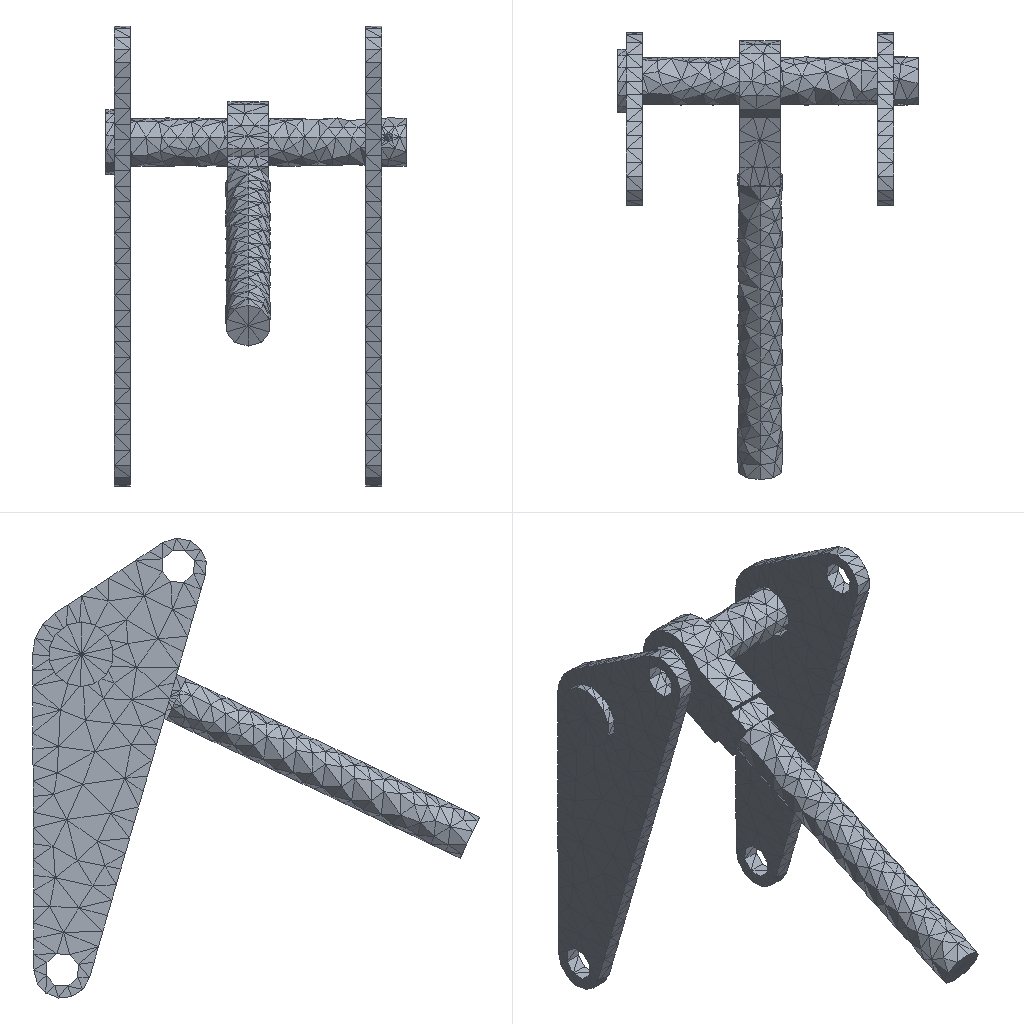Simulation study | ansys workbench
Ansys APDL input file, long lists of numbers shortened:
/batch
/config,noeldb,1     ! force off writing results to database
*get,_wallstrt,active,,time,wall
! ANSYS input file written by Workbench version 2022 R1
! File used for geometry attach:
/title,0-0--____ (C5)
! ****** Begin Custom Load Command Snippet ******
/COM, ACT Extensions:
/COM,     LSDYNA, 2021.1
/COM,
! ****** End   Custom Load Command Snippet ******
*DIM,_wb_ProjectScratch_dir,string,248
_wb_ProjectScratch_dir(1) = ''
*DIM,_wb_SolverFiles_dir,string,248
_wb_SolverFiles_dir(1) = ''
*DIM,_wb_userfiles_dir,string,248
_wb_userfiles_dir(1) = ''
/com,--- Data in consistent NMM units. See Solving Units in the help system for more information.
/units,MPA
/nopr
/wb,file,start              !  signify a WB generated input file
/prep7
! Turn off shape checking because checks already performed inside WB mesher.
! See help system for more information.
SHPP,OFF,,NOWARN
/nolist
etcon,set             ! allow ANSYS to choose best KEYOP's for 180x elements, resets any applicable keyopt to MAPDL defaults
/com,*********** Nodes for the whole assembly ***********
nblock,3,,7470
(1i9,3e20.9e3)
        1    -2.013006712E+02     4.007910257E+02    -4.722712683E+02
! (6790 more lines like these left out)
-1
/wb,elem,start            !  set before creation of elements
/com,*********** Elements for Body 1 "__28__250|____-____2" ***********
et,1,187
eblock,19,solid,,1096
(19i9)
        1        1        1        1        0        0        0        0       10        0        1       96      399      165      348     1032     1339     1025     1029
! (2191 more lines like these left out)
-1
/com,*********** Elements for Body 2 "__1|____-____1" ***********
et,2,187
eblock,19,solid,,568
(19i9)
        2        2        2        2        0        0        0        0       10        0     2588     5542     5693     5558     5617     6303     6356     6300     6302
! (1135 more lines like these left out)
-1
/com,*********** Elements for Body 3 "__1|____-____1[2]" ***********
et,3,187
eblock,19,solid,,568
(19i9)
        3        3        3        3        0        0        0        0       10        0     2020     4177     4328     4193     4252     4938     4991     4935     4937
! (1135 more lines like these left out)
-1
/com,*********** Elements for Body 4 "M30X180__|____-____1" ***********
et,4,187
eblock,19,solid,,923
(19i9)
        4        4        4        4        0        0        0        0       10        0     1097     2363     2557     2533     2548     3258     4046     3256     3257
! (1845 more lines like these left out)
-1
/wb,elem,end               !  done creating elements
/com,*********** Send User Defined Coordinate System(s) ***********
csys,0
toffst,273.15,  ! Temperature offset from absolute zero
/com,*********** Set Reference Temperature ***********
tref,22.
/wb,mat,start              !  starting to send materials
/com,*********** Send Materials ***********
Temperature = 'TEMP' ! Temperature
MP,DENS,1,7.85e-09,	! tonne mm^-3
MP,ALPX,1,1.2e-05,	! C^-1
MP,C,1,434000000,	! mm^2 s^-2 C^-1
MP,KXX,1,60.5,	! tonne mm s^-3 C^-1
MP,RSVX,1,0.00017,	! ohm mm
MP,EX,1,200000,	! tonne s^-2 mm^-1
MP,NUXY,1,0.3,
MP,MURX,1,10000,
Temperature = 'TEMP' ! Temperature
MP,DENS,2,7.85e-09,	! tonne mm^-3
MP,ALPX,2,1.2e-05,	! C^-1
MP,C,2,434000000,	! mm^2 s^-2 C^-1
MP,KXX,2,60.5,	! tonne mm s^-3 C^-1
MP,RSVX,2,0.00017,	! ohm mm
MP,EX,2,200000,	! tonne s^-2 mm^-1
MP,NUXY,2,0.3,
MP,MURX,2,10000,
Temperature = 'TEMP' ! Temperature
MP,DENS,3,7.85e-09,	! tonne mm^-3
MP,ALPX,3,1.2e-05,	! C^-1
MP,C,3,434000000,	! mm^2 s^-2 C^-1
MP,KXX,3,60.5,	! tonne mm s^-3 C^-1
MP,RSVX,3,0.00017,	! ohm mm
MP,EX,3,200000,	! tonne s^-2 mm^-1
MP,NUXY,3,0.3,
MP,MURX,3,10000,
Temperature = 'TEMP' ! Temperature
MP,DENS,4,7.85e-09,	! tonne mm^-3
MP,ALPX,4,1.2e-05,	! C^-1
MP,C,4,434000000,	! mm^2 s^-2 C^-1
MP,KXX,4,60.5,	! tonne mm s^-3 C^-1
MP,RSVX,4,0.00017,	! ohm mm
MP,EX,4,200000,	! tonne s^-2 mm^-1
MP,NUXY,4,0.3,
MP,MURX,4,10000,
/wb,mat,end                !  done sending materials
!************************* Model Summary ********************
!__28__250|____-____2,	结构钢,	matid,	1
!__1|____-____1,	结构钢,	matid,	2
!__1|____-____1[2],	结构钢,	matid,	3
!M30X180__|____-____1,	结构钢,	matid,	4
!************************* End Model Summary ********************
! get the diagonal of the bounding box. Needed later for other things
*get,_xmin,node,,mnloc,x
*get,_ymin,node,,mnloc,y
*get,_zmin,node,,mnloc,z
*get,_xmax,node,,mxloc,x
*get,_ymax,node,,mxloc,y
*get,_zmax,node,,mxloc,z
_ASMDIAG=(_xmax-_xmin)*(_xmax-_xmin)+(_ymax-_ymin)*(_ymax-_ymin)+(_zmax-_zmin)*(_zmax-_zmin)
_ASMDIAG=SQRT(_ASMDIAG)
/wb,contact,start          !  starting to send contact
/com,*********** Create Contact "摩擦的 - 杆径28行程250|____-____2 至 M30X180销轴|____-____1" ***********
/com,            Real Constant Set For Above Contact Is 6 & 5
*set,tid,6
*set,cid,5
r,tid
r,cid
et,tid,170
et,cid,174
eblock,10,,,48
(15i9)
     5424        6        6        6        0        8        9      328      328      450      462      328      453
! (47 more lines like these left out)
-1
eblock,10,,,48
(15i9)
     5472        5        5        5        0        8        9      328      328      450      462      328      453
! (47 more lines like these left out)
-1
eblock,10,,,96
(15i9)
     5520        5        6        5        0     2290     2291     2450     2450     2832     2843     2450     2836
! (95 more lines like these left out)
-1
eblock,10,,,96
(15i9)
     5616        6        5        6        0     2290     2291     2450     2450     2832     2843     2450     2836
! (95 more lines like these left out)
-1
keyo,cid,8,2               ! auto create asymmetric contact (from Program Controlled setting)
keyo,cid,10,0              ! adjust contact stiffness each NR iteration (from Program Controlled setting)
keyo,cid,12,0              ! standard contact
mp,mu,cid,0.3       ! unitless
keyo,cid,18,1              ! small sliding turned on by application
keyo,cid,2,0               ! augmented Lagrange (from Program Controlled setting)
keyo,cid,4,0               ! on Gauss point (from Program Controlled setting)
keyo,cid,9,0               ! use real geometry with stepped effects
keyo,cid,7,0               ! No Prediction
rmod,tid,3,1.       ! FKN
rmod,tid,5,0.       ! ICONT
rmod,tid,6,0.       ! PINB
rmod,tid,10,0.      ! CNOF
rmod,tid,12,0.      ! FKT
rmod,tid,36,35      ! WB DSID
rmod,cid,3,1.       ! FKN
rmod,cid,5,0.       ! ICONT
rmod,cid,6,0.       ! PINB
rmod,cid,10,0.      ! CNOF
rmod,cid,12,0.      ! FKT
rmod,cid,36,35      ! WB DSID
/com,*********** Create Contact "绑定 - M30X180销轴|____-____1 至 多个" ***********
/com,            Real Constant Set For Above Contact Is 8 & 7
*set,tid,8
*set,cid,7
r,tid
r,cid
et,tid,170
et,cid,174
eblock,10,,,404
(15i9)
     5712        8        8        8        0     2319     2318     2349     2349     3040     3043     2349     3049
! (403 more lines like these left out)
-1
eblock,10,,,404
(15i9)
     6116        7        7        7        0     2319     2318     2349     2349     3040     3043     2349     3049
! (403 more lines like these left out)
-1
eblock,10,,,48
(15i9)
     6520        7        8        7        0     5437     5439     5445     5445     5756     5771     5445     5757
! (47 more lines like these left out)
-1
eblock,10,,,48
(15i9)
     6568        8        7        8        0     5437     5439     5445     5445     5756     5771     5445     5757
! (47 more lines like these left out)
-1
keyo,cid,8,2               ! auto create asymmetric contact (from Program Controlled setting)
keyo,cid,10,0              ! adjust contact stiffness each NR iteration (from Program Controlled setting)
keyo,cid,12,5              ! bonded always
keyo,cid,2,2               ! MPC contact.  Valid only for bonded or no separation.  Requires nodal detection
keyo,cid,4,2               ! on nodal point - normal to target surface (from Program Controlled setting)
keyo,cid,9,1               ! ignore initial gaps/penetration
keyo,cid,7,0               ! No Prediction
rmod,tid,3,1.       ! FKN
rmod,tid,5,0.       ! ICONT
rmod,tid,6,0.       ! PINB
rmod,tid,10,0.      ! CNOF
rmod,tid,12,0.      ! FKT
rmod,tid,36,38      ! WB DSID
rmod,cid,3,1.       ! FKN
rmod,cid,5,0.       ! ICONT
rmod,cid,6,0.       ! PINB
rmod,cid,10,0.      ! CNOF
rmod,cid,12,0.      ! FKT
rmod,cid,36,38      ! WB DSID
nsel,all
esel,all
/wb,contact,end            !  done creating contacts
/golist
/wb,load,start             !  starting to send loads
/com,*********** Fixed Supports ***********
CMBLOCK,_FIXEDSU,NODE,      108
(8i10)
      4062      4063      4064      4065      4066      4067      4068      4069
! (13 more lines like these left out)
cmsel,s,_FIXEDSU
d,all,all
nsel,all
/com,*********** Define Force Using Surface Effect Elements ***********
local,12,0,0.,0.,0.,0.,0.,0.
csys,0
et,9,154
eblock,10,,,60
(15i9)
     6616        9        9        9       12       33       18       23       23      528      527       23      546
! (59 more lines like these left out)
-1
esel,s,type,,9
keyop,9,2,1                ! Apply load in local coordinate system
keyop,9,7,1                ! Use original area so load is constant in large deformation
esel,all
/gst,on,on
fini
*get,_numnode,node,0,count
*get,_numelem,elem,0,count
*get, _MAXELEMNUM, elem, 0, NUM, MAX
*get, _MAXNODENUM, node, 0, NUM, MAX
*get, _MAXELEMTYPE, etyp, 0, NUM, MAX
*get, _MAXREALCONST, real, 0, NUM, MAX
/go
/wb,load,end               !  done creating loads
/com,--- Number of total nodes = %_numnode%
/com,--- Number of contact elements = 1252
/com,--- Number of spring elements = 0
/com,--- Number of bearing elements = 0
/com,--- Number of solid elements = 3155
/com,--- Number of condensed parts = 0
/com,--- Number of total elements = %_numelem%
*get,_wallbsol,active,,time,wall
/com,****************************************************************************
/com,*************************    SOLUTION       ********************************
/com,****************************************************************************
/solu
antype,0                   ! static analysis
_thickRatio=0.5     ! Ratio of thick parts in the model
eqsl,sparse,,,,,1
cntr,print,1               ! print out contact info and also make no initial contact an error
dmpoption,emat,no             ! Don't combine emat file for DANSYS
dmpoption,esav,no             ! Don't combine esav file for DANSYS
nldiag,cont,iter           ! print out contact info each equilibrium iteration
rescontrol,define,last,last,,dele	   ! Program Controlled
/com,****************************************************
/com,******************* SOLVE FOR LS 1 OF 1 ****************
esel,s,type,,9
nsle
sfe,all,1,pres,1,0.
sfe,all,2,pres,1,9.527
sfe,all,3,pres,1,4.496
nsel,all
esel,all
/nopr
/gopr
autots,on                  ! Workbench Program Controlled automatic time stepping
nsub,5,20,1                ! due to presence of high frictional contact
time,1.
outres,erase
outres,all,none
outres,nsol,all,
outres,rsol,all
outres,eangl,all
outres,etmp,all
outres,veng,all
outres,strs,all,
outres,epel,all,
outres,eppl,all,
outres,cont,all,
! *********** WB SOLVE COMMAND ***********
! check interactive state
*get,ANSINTER_,active,,int
*if,ANSINTER_,ne,0,then
/eof
*endif
solve
/com *************** Write FE CONNECTORS *********
CEWRITE,file,ce,,INTE
/com,****************************************************
/com,*************** FINISHED SOLVE FOR LS 1 *************
*get,_wallasol,active,,time,wall
/nopr
*get,_numnode,node,0,count
*get,_numelem,elem,0,count
*get, _MAXELEMNUM, elem, 0, NUM, MAX
*get, _MAXNODENUM, node, 0, NUM, MAX,,,INTERNAL
*get, _MAXELEMTYPE, etyp, 0, NUM, MAX
*get, _MAXREALCONST, real, 0, NUM, MAX
/gopr
/post1
xmlo,ENCODING,ISO-8859-1
xmlo,parm
/xml,parm,xml
fini
/gopr
*get,_walldone,active,,time,wall
_preptime=(_wallbsol-_wallstrt)*3600
_solvtime=(_wallasol-_wallbsol)*3600
_posttime=(_walldone-_wallasol)*3600
_totaltim=(_walldone-_wallstrt)*3600
*get,_dlbratio,active,0,solu,dlbr
*get,_combtime,active,0,solu,comb
*get,_ssmode,active,0,solu,ssmm
*get,_ndofs,active,0,solu,ndof
*get,_sol_end_time,active,0,set,time
*if,_sol_end_time,eq,1.,then
/fclean				!clean distributed files
*endif
/com,--- Total number of nodes = %_numnode%
/com,--- Total number of elements = %_numelem%
/com,--- Element load balance ratio = %_dlbratio%
/com,--- Time to combine distributed files = %_combtime%
/com,--- Sparse memory mode = %_ssmode%
/com,--- Number of DOF = %_ndofs%
/wb,file,end               ! done with WB generated input